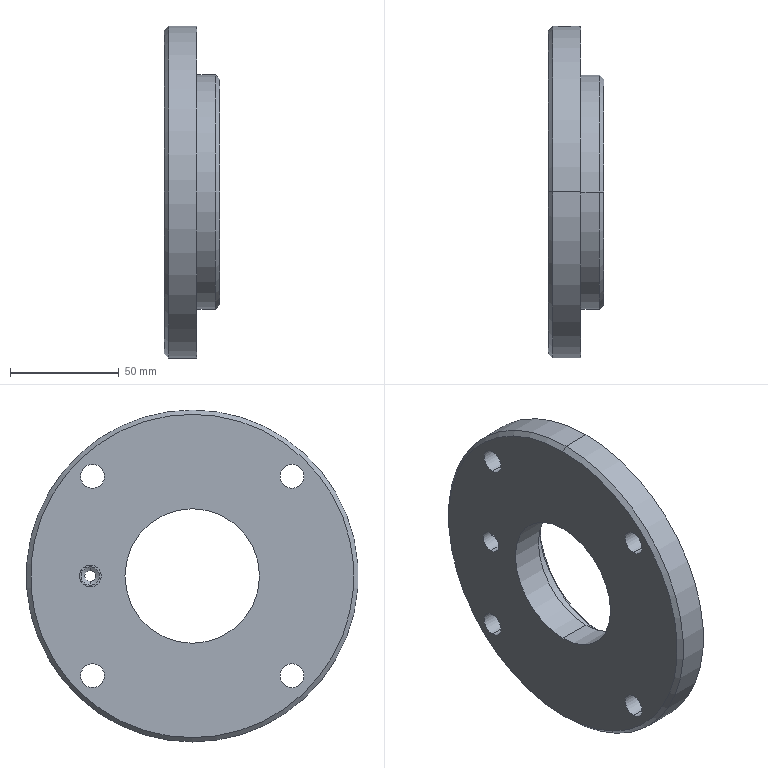Part | STEP file | Input 20 | 1 solid | 44 faces | box 25.5 x 153 x 153 mm | volume 263994 mm3 | cylinder 28 | cone 8 | plane 6 | torus 2 | commonest cylinder face diameters 11 x8 5 x4 8.5 x4 10 x4 62 x2 80 x2